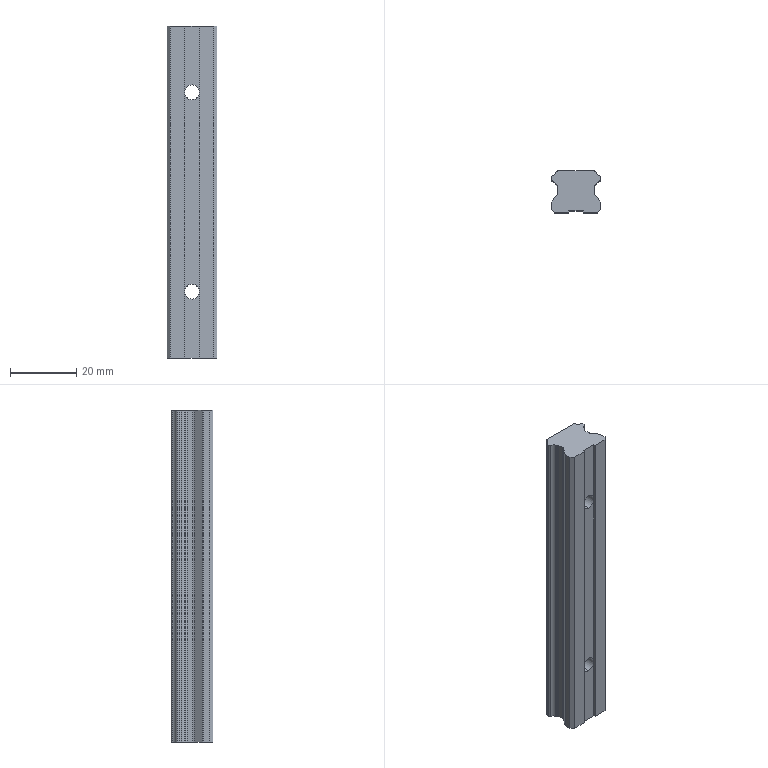Part | SolidWorks | features 3DProfileFeature 1, Extrusion 1, HoleWzd 1, LPattern 1 | 1 solid | 50 faces | box 15 x 12.5 x 100 mm | volume 15532 mm3 | cylinder 26 | plane 24 | commonest cylinder face diameters 1 x12 3 x4 4.5 x4 8 x4 2 x2